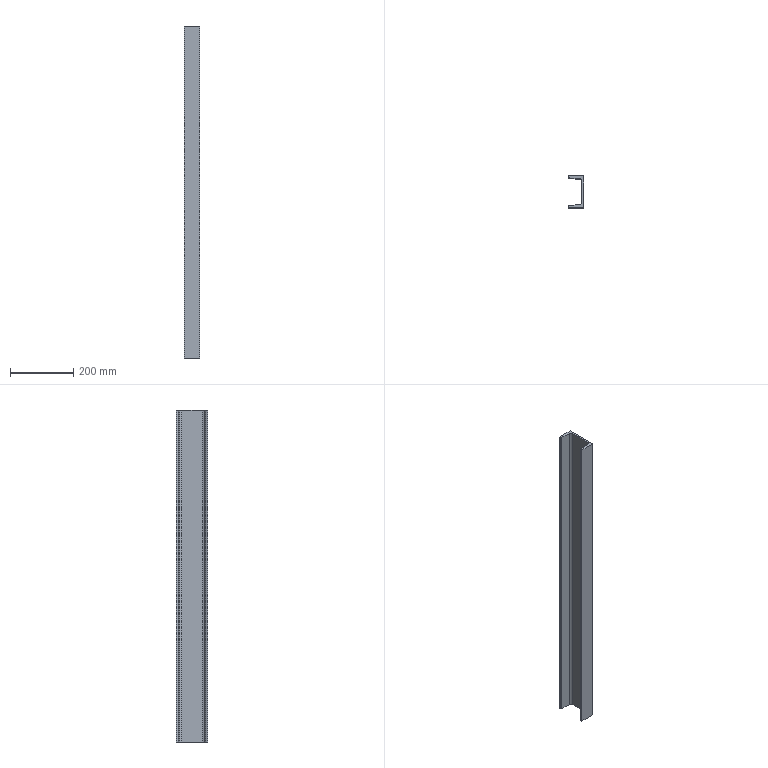Part | SolidWorks | features BaseBody 1 | 1 solid | 14 faces | box 48 x 100 x 1046 mm | volume 1315987 mm3 | plane 10 | cylinder 4 | commonest cylinder face diameters 8.5 x2 17 x2
STEP:
#1=CARTESIAN_POINT('',(2.65,50.,-523.));
#2=VERTEX_POINT('',#1);
#3=CARTESIAN_POINT('',(2.65,-50.,-523.));
#4=VERTEX_POINT('',#3);
#5=CARTESIAN_POINT('',(2.65,50.,-523.));
#6=DIRECTION('',(0.,-1.,0.));
#7=VECTOR('',#6,1000.);
#8=LINE('',#5,#7);
#9=EDGE_CURVE('',#2,#4,#8,.T.);
#10=ORIENTED_EDGE('',*,*,#9,.T.);
#11=CARTESIAN_POINT('',(-45.35,-50.,-523.));
#12=VERTEX_POINT('',#11);
#13=CARTESIAN_POINT('',(2.65,-50.,-523.));
#14=DIRECTION('',(-1.,0.,0.));
#15=VECTOR('',#14,1000.);
#16=LINE('',#13,#15);
#17=EDGE_CURVE('',#4,#12,#16,.T.);
#18=ORIENTED_EDGE('',*,*,#17,.T.);
#19=CARTESIAN_POINT('',(-45.35,-47.266,-523.));
#20=VERTEX_POINT('',#19);
#21=CARTESIAN_POINT('',(-45.35,-47.266,-523.));
#22=DIRECTION('',(0.,-1.,0.));
#23=VECTOR('',#22,1000.);
#24=LINE('',#21,#23);
#25=EDGE_CURVE('',#20,#12,#24,.T.);
#26=ORIENTED_EDGE('',*,*,#25,.F.);
#27=CARTESIAN_POINT('',(-41.423,-43.028,-523.));
#28=VERTEX_POINT('',#27);
#29=CARTESIAN_POINT('',(-41.1,-47.266,-523.));
#30=DIRECTION('',(0.,0.,1.));
#31=DIRECTION('',(1.,0.,0.));
#32=AXIS2_PLACEMENT_3D('',#29,#30,#31);
#33=CIRCLE('',#32,4.25);
#34=EDGE_CURVE('',#28,#20,#33,.T.);
#35=ORIENTED_EDGE('',*,*,#34,.F.);
#36=CARTESIAN_POINT('',(-10.505,-40.675,-523.));
#37=VERTEX_POINT('',#36);
#38=CARTESIAN_POINT('',(-10.505,-40.675,-523.));
#39=DIRECTION('',(-0.9971,-0.07589,0.));
#40=VECTOR('',#39,1000.);
#41=LINE('',#38,#40);
#42=EDGE_CURVE('',#37,#28,#41,.T.);
#43=ORIENTED_EDGE('',*,*,#42,.F.);
#44=CARTESIAN_POINT('',(-2.65,-32.199,-523.));
#45=VERTEX_POINT('',#44);
#46=CARTESIAN_POINT('',(-11.15,-32.199,-523.));
#47=DIRECTION('',(0.,0.,-1.));
#48=DIRECTION('',(-1.,0.,0.));
#49=AXIS2_PLACEMENT_3D('',#46,#47,#48);
#50=CIRCLE('',#49,8.5);
#51=EDGE_CURVE('',#45,#37,#50,.T.);
#52=ORIENTED_EDGE('',*,*,#51,.F.);
#53=CARTESIAN_POINT('',(-2.65,32.199,-523.));
#54=VERTEX_POINT('',#53);
#55=CARTESIAN_POINT('',(-2.65,-32.199,-523.));
#56=DIRECTION('',(0.,1.,0.));
#57=VECTOR('',#56,1000.);
#58=LINE('',#55,#57);
#59=EDGE_CURVE('',#45,#54,#58,.T.);
#60=ORIENTED_EDGE('',*,*,#59,.T.);
#61=CARTESIAN_POINT('',(-10.505,40.675,-523.));
#62=VERTEX_POINT('',#61);
#63=CARTESIAN_POINT('',(-11.15,32.199,-523.));
#64=DIRECTION('',(0.,0.,-1.));
#65=DIRECTION('',(-1.,0.,0.));
#66=AXIS2_PLACEMENT_3D('',#63,#64,#65);
#67=CIRCLE('',#66,8.5);
#68=EDGE_CURVE('',#62,#54,#67,.T.);
#69=ORIENTED_EDGE('',*,*,#68,.F.);
#70=CARTESIAN_POINT('',(-41.423,43.028,-523.));
#71=VERTEX_POINT('',#70);
#72=CARTESIAN_POINT('',(-10.505,40.675,-523.));
#73=DIRECTION('',(-0.9971,0.07589,0.));
#74=VECTOR('',#73,1000.);
#75=LINE('',#72,#74);
#76=EDGE_CURVE('',#62,#71,#75,.T.);
#77=ORIENTED_EDGE('',*,*,#76,.T.);
#78=CARTESIAN_POINT('',(-45.35,47.266,-523.));
#79=VERTEX_POINT('',#78);
#80=CARTESIAN_POINT('',(-41.1,47.266,-523.));
#81=DIRECTION('',(0.,0.,1.));
#82=DIRECTION('',(1.,0.,0.));
#83=AXIS2_PLACEMENT_3D('',#80,#81,#82);
#84=CIRCLE('',#83,4.25);
#85=EDGE_CURVE('',#79,#71,#84,.T.);
#86=ORIENTED_EDGE('',*,*,#85,.F.);
#87=CARTESIAN_POINT('',(-45.35,50.,-523.));
#88=VERTEX_POINT('',#87);
#89=CARTESIAN_POINT('',(-45.35,47.266,-523.));
#90=DIRECTION('',(0.,1.,0.));
#91=VECTOR('',#90,1000.);
#92=LINE('',#89,#91);
#93=EDGE_CURVE('',#79,#88,#92,.T.);
#94=ORIENTED_EDGE('',*,*,#93,.T.);
#95=CARTESIAN_POINT('',(2.65,50.,-523.));
#96=DIRECTION('',(-1.,0.,0.));
#97=VECTOR('',#96,1000.);
#98=LINE('',#95,#97);
#99=EDGE_CURVE('',#2,#88,#98,.T.);
#100=ORIENTED_EDGE('',*,*,#99,.F.);
#101=EDGE_LOOP('',(#10,#18,#26,#35,#43,#52,#60,#69,#77,#86,#94,#100));
#102=FACE_OUTER_BOUND('',#101,.T.);
#103=CARTESIAN_POINT('',(-41.1,-47.266,-523.));
#104=DIRECTION('',(0.,0.,1.));
#105=DIRECTION('',(1.,0.,0.));
#106=AXIS2_PLACEMENT_3D('',#103,#104,#105);
#107=PLANE('',#106);
#108=ADVANCED_FACE('',(#102),#107,.F.);
#109=CARTESIAN_POINT('',(2.65,50.,523.));
#110=VERTEX_POINT('',#109);
#111=CARTESIAN_POINT('',(2.65,-50.,523.));
#112=VERTEX_POINT('',#111);
#113=CARTESIAN_POINT('',(2.65,50.,523.));
#114=DIRECTION('',(0.,-1.,0.));
#115=VECTOR('',#114,1000.);
#116=LINE('',#113,#115);
#117=EDGE_CURVE('',#110,#112,#116,.T.);
#118=ORIENTED_EDGE('',*,*,#117,.F.);
#119=CARTESIAN_POINT('',(-45.35,50.,523.));
#120=VERTEX_POINT('',#119);
#121=CARTESIAN_POINT('',(2.65,50.,523.));
#122=DIRECTION('',(-1.,0.,0.));
#123=VECTOR('',#122,1000.);
#124=LINE('',#121,#123);
#125=EDGE_CURVE('',#110,#120,#124,.T.);
#126=ORIENTED_EDGE('',*,*,#125,.T.);
#127=CARTESIAN_POINT('',(-45.35,47.266,523.));
#128=VERTEX_POINT('',#127);
#129=CARTESIAN_POINT('',(-45.35,47.266,523.));
#130=DIRECTION('',(0.,1.,0.));
#131=VECTOR('',#130,1000.);
#132=LINE('',#129,#131);
#133=EDGE_CURVE('',#128,#120,#132,.T.);
#134=ORIENTED_EDGE('',*,*,#133,.F.);
#135=CARTESIAN_POINT('',(-41.423,43.028,523.));
#136=VERTEX_POINT('',#135);
#137=CARTESIAN_POINT('',(-41.1,47.266,523.));
#138=DIRECTION('',(0.,0.,1.));
#139=DIRECTION('',(1.,0.,0.));
#140=AXIS2_PLACEMENT_3D('',#137,#138,#139);
#141=CIRCLE('',#140,4.25);
#142=EDGE_CURVE('',#128,#136,#141,.T.);
#143=ORIENTED_EDGE('',*,*,#142,.T.);
#144=CARTESIAN_POINT('',(-10.505,40.675,523.));
#145=VERTEX_POINT('',#144);
#146=CARTESIAN_POINT('',(-10.505,40.675,523.));
#147=DIRECTION('',(-0.9971,0.07589,0.));
#148=VECTOR('',#147,1000.);
#149=LINE('',#146,#148);
#150=EDGE_CURVE('',#145,#136,#149,.T.);
#151=ORIENTED_EDGE('',*,*,#150,.F.);
#152=CARTESIAN_POINT('',(-2.65,32.199,523.));
#153=VERTEX_POINT('',#152);
#154=CARTESIAN_POINT('',(-11.15,32.199,523.));
#155=DIRECTION('',(0.,0.,-1.));
#156=DIRECTION('',(-1.,0.,0.));
#157=AXIS2_PLACEMENT_3D('',#154,#155,#156);
#158=CIRCLE('',#157,8.5);
#159=EDGE_CURVE('',#145,#153,#158,.T.);
#160=ORIENTED_EDGE('',*,*,#159,.T.);
#161=CARTESIAN_POINT('',(-2.65,-32.199,523.));
#162=VERTEX_POINT('',#161);
#163=CARTESIAN_POINT('',(-2.65,-32.199,523.));
#164=DIRECTION('',(0.,1.,0.));
#165=VECTOR('',#164,1000.);
#166=LINE('',#163,#165);
#167=EDGE_CURVE('',#162,#153,#166,.T.);
#168=ORIENTED_EDGE('',*,*,#167,.F.);
#169=CARTESIAN_POINT('',(-10.505,-40.675,523.));
#170=VERTEX_POINT('',#169);
#171=CARTESIAN_POINT('',(-11.15,-32.199,523.));
#172=DIRECTION('',(0.,0.,-1.));
#173=DIRECTION('',(-1.,0.,0.));
#174=AXIS2_PLACEMENT_3D('',#171,#172,#173);
#175=CIRCLE('',#174,8.5);
#176=EDGE_CURVE('',#162,#170,#175,.T.);
#177=ORIENTED_EDGE('',*,*,#176,.T.);
#178=CARTESIAN_POINT('',(-41.423,-43.028,523.));
#179=VERTEX_POINT('',#178);
#180=CARTESIAN_POINT('',(-10.505,-40.675,523.));
#181=DIRECTION('',(-0.9971,-0.07589,0.));
#182=VECTOR('',#181,1000.);
#183=LINE('',#180,#182);
#184=EDGE_CURVE('',#170,#179,#183,.T.);
#185=ORIENTED_EDGE('',*,*,#184,.T.);
#186=CARTESIAN_POINT('',(-45.35,-47.266,523.));
#187=VERTEX_POINT('',#186);
#188=CARTESIAN_POINT('',(-41.1,-47.266,523.));
#189=DIRECTION('',(0.,0.,1.));
#190=DIRECTION('',(1.,0.,0.));
#191=AXIS2_PLACEMENT_3D('',#188,#189,#190);
#192=CIRCLE('',#191,4.25);
#193=EDGE_CURVE('',#179,#187,#192,.T.);
#194=ORIENTED_EDGE('',*,*,#193,.T.);
#195=CARTESIAN_POINT('',(-45.35,-50.,523.));
#196=VERTEX_POINT('',#195);
#197=CARTESIAN_POINT('',(-45.35,-47.266,523.));
#198=DIRECTION('',(0.,-1.,0.));
#199=VECTOR('',#198,1000.);
#200=LINE('',#197,#199);
#201=EDGE_CURVE('',#187,#196,#200,.T.);
#202=ORIENTED_EDGE('',*,*,#201,.T.);
#203=CARTESIAN_POINT('',(2.65,-50.,523.));
#204=DIRECTION('',(-1.,0.,0.));
#205=VECTOR('',#204,1000.);
#206=LINE('',#203,#205);
#207=EDGE_CURVE('',#112,#196,#206,.T.);
#208=ORIENTED_EDGE('',*,*,#207,.F.);
#209=EDGE_LOOP('',(#118,#126,#134,#143,#151,#160,#168,#177,#185,#194,#202,#208));
#210=FACE_OUTER_BOUND('',#209,.T.);
#211=CARTESIAN_POINT('',(-41.1,-47.266,523.));
#212=DIRECTION('',(0.,0.,1.));
#213=DIRECTION('',(1.,0.,0.));
#214=AXIS2_PLACEMENT_3D('',#211,#212,#213);
#215=PLANE('',#214);
#216=ADVANCED_FACE('',(#210),#215,.T.);
#217=ORIENTED_EDGE('',*,*,#17,.F.);
#218=CARTESIAN_POINT('',(2.65,-50.,523.));
#219=DIRECTION('',(0.,0.,-1.));
#220=VECTOR('',#219,1000.);
#221=LINE('',#218,#220);
#222=EDGE_CURVE('',#112,#4,#221,.T.);
#223=ORIENTED_EDGE('',*,*,#222,.F.);
#224=ORIENTED_EDGE('',*,*,#207,.T.);
#225=CARTESIAN_POINT('',(-45.35,-50.,523.));
#226=DIRECTION('',(0.,0.,-1.));
#227=VECTOR('',#226,1000.);
#228=LINE('',#225,#227);
#229=EDGE_CURVE('',#196,#12,#228,.T.);
#230=ORIENTED_EDGE('',*,*,#229,.T.);
#231=EDGE_LOOP('',(#217,#223,#224,#230));
#232=FACE_OUTER_BOUND('',#231,.T.);
#233=CARTESIAN_POINT('',(2.65,-50.,523.));
#234=DIRECTION('',(0.,-1.,0.));
#235=DIRECTION('',(0.,0.,-1.));
#236=AXIS2_PLACEMENT_3D('',#233,#234,#235);
#237=PLANE('',#236);
#238=ADVANCED_FACE('',(#232),#237,.T.);
#239=ORIENTED_EDGE('',*,*,#25,.T.);
#240=ORIENTED_EDGE('',*,*,#229,.F.);
#241=ORIENTED_EDGE('',*,*,#201,.F.);
#242=CARTESIAN_POINT('',(-45.35,-47.266,523.));
#243=DIRECTION('',(0.,0.,-1.));
#244=VECTOR('',#243,1000.);
#245=LINE('',#242,#244);
#246=EDGE_CURVE('',#187,#20,#245,.T.);
#247=ORIENTED_EDGE('',*,*,#246,.T.);
#248=EDGE_LOOP('',(#239,#240,#241,#247));
#249=FACE_OUTER_BOUND('',#248,.T.);
#250=CARTESIAN_POINT('',(-45.35,-47.266,523.));
#251=DIRECTION('',(1.,0.,0.));
#252=DIRECTION('',(0.,1.,0.));
#253=AXIS2_PLACEMENT_3D('',#250,#251,#252);
#254=PLANE('',#253);
#255=ADVANCED_FACE('',(#249),#254,.F.);
#256=ORIENTED_EDGE('',*,*,#34,.T.);
#257=ORIENTED_EDGE('',*,*,#246,.F.);
#258=ORIENTED_EDGE('',*,*,#193,.F.);
#259=CARTESIAN_POINT('',(-41.423,-43.028,523.));
#260=DIRECTION('',(0.,0.,-1.));
#261=VECTOR('',#260,1000.);
#262=LINE('',#259,#261);
#263=EDGE_CURVE('',#179,#28,#262,.T.);
#264=ORIENTED_EDGE('',*,*,#263,.T.);
#265=EDGE_LOOP('',(#256,#257,#258,#264));
#266=FACE_OUTER_BOUND('',#265,.T.);
#267=CARTESIAN_POINT('',(-41.1,-47.266,523.));
#268=DIRECTION('',(0.,0.,-1.));
#269=DIRECTION('',(-1.,0.,0.));
#270=AXIS2_PLACEMENT_3D('',#267,#268,#269);
#271=CYLINDRICAL_SURFACE('',#270,4.25);
#272=ADVANCED_FACE('',(#266),#271,.T.);
#273=ORIENTED_EDGE('',*,*,#42,.T.);
#274=ORIENTED_EDGE('',*,*,#263,.F.);
#275=ORIENTED_EDGE('',*,*,#184,.F.);
#276=CARTESIAN_POINT('',(-10.505,-40.675,523.));
#277=DIRECTION('',(0.,0.,-1.));
#278=VECTOR('',#277,1000.);
#279=LINE('',#276,#278);
#280=EDGE_CURVE('',#170,#37,#279,.T.);
#281=ORIENTED_EDGE('',*,*,#280,.T.);
#282=EDGE_LOOP('',(#273,#274,#275,#281));
#283=FACE_OUTER_BOUND('',#282,.T.);
#284=CARTESIAN_POINT('',(-10.505,-40.675,523.));
#285=DIRECTION('',(0.07589,-0.9971,0.));
#286=DIRECTION('',(0.,0.,-1.));
#287=AXIS2_PLACEMENT_3D('',#284,#285,#286);
#288=PLANE('',#287);
#289=ADVANCED_FACE('',(#283),#288,.F.);
#290=ORIENTED_EDGE('',*,*,#51,.T.);
#291=ORIENTED_EDGE('',*,*,#280,.F.);
#292=ORIENTED_EDGE('',*,*,#176,.F.);
#293=CARTESIAN_POINT('',(-2.65,-32.199,523.));
#294=DIRECTION('',(0.,0.,-1.));
#295=VECTOR('',#294,1000.);
#296=LINE('',#293,#295);
#297=EDGE_CURVE('',#162,#45,#296,.T.);
#298=ORIENTED_EDGE('',*,*,#297,.T.);
#299=EDGE_LOOP('',(#290,#291,#292,#298));
#300=FACE_OUTER_BOUND('',#299,.T.);
#301=CARTESIAN_POINT('',(-11.15,-32.199,523.));
#302=DIRECTION('',(0.,0.,-1.));
#303=DIRECTION('',(-1.,0.,0.));
#304=AXIS2_PLACEMENT_3D('',#301,#302,#303);
#305=CYLINDRICAL_SURFACE('',#304,8.5);
#306=ADVANCED_FACE('',(#300),#305,.F.);
#307=ORIENTED_EDGE('',*,*,#59,.F.);
#308=ORIENTED_EDGE('',*,*,#297,.F.);
#309=ORIENTED_EDGE('',*,*,#167,.T.);
#310=CARTESIAN_POINT('',(-2.65,32.199,523.));
#311=DIRECTION('',(0.,0.,-1.));
#312=VECTOR('',#311,1000.);
#313=LINE('',#310,#312);
#314=EDGE_CURVE('',#153,#54,#313,.T.);
#315=ORIENTED_EDGE('',*,*,#314,.T.);
#316=EDGE_LOOP('',(#307,#308,#309,#315));
#317=FACE_OUTER_BOUND('',#316,.T.);
#318=CARTESIAN_POINT('',(-2.65,-32.199,523.));
#319=DIRECTION('',(-1.,0.,0.));
#320=DIRECTION('',(0.,1.,0.));
#321=AXIS2_PLACEMENT_3D('',#318,#319,#320);
#322=PLANE('',#321);
#323=ADVANCED_FACE('',(#317),#322,.T.);
#324=ORIENTED_EDGE('',*,*,#68,.T.);
#325=ORIENTED_EDGE('',*,*,#314,.F.);
#326=ORIENTED_EDGE('',*,*,#159,.F.);
#327=CARTESIAN_POINT('',(-10.505,40.675,523.));
#328=DIRECTION('',(0.,0.,-1.));
#329=VECTOR('',#328,1000.);
#330=LINE('',#327,#329);
#331=EDGE_CURVE('',#145,#62,#330,.T.);
#332=ORIENTED_EDGE('',*,*,#331,.T.);
#333=EDGE_LOOP('',(#324,#325,#326,#332));
#334=FACE_OUTER_BOUND('',#333,.T.);
#335=CARTESIAN_POINT('',(-11.15,32.199,523.));
#336=DIRECTION('',(0.,0.,-1.));
#337=DIRECTION('',(-1.,0.,0.));
#338=AXIS2_PLACEMENT_3D('',#335,#336,#337);
#339=CYLINDRICAL_SURFACE('',#338,8.5);
#340=ADVANCED_FACE('',(#334),#339,.F.);
#341=ORIENTED_EDGE('',*,*,#76,.F.);
#342=ORIENTED_EDGE('',*,*,#331,.F.);
#343=ORIENTED_EDGE('',*,*,#150,.T.);
#344=CARTESIAN_POINT('',(-41.423,43.028,523.));
#345=DIRECTION('',(0.,0.,-1.));
#346=VECTOR('',#345,1000.);
#347=LINE('',#344,#346);
#348=EDGE_CURVE('',#136,#71,#347,.T.);
#349=ORIENTED_EDGE('',*,*,#348,.T.);
#350=EDGE_LOOP('',(#341,#342,#343,#349));
#351=FACE_OUTER_BOUND('',#350,.T.);
#352=CARTESIAN_POINT('',(-10.505,40.675,523.));
#353=DIRECTION('',(-0.07589,-0.9971,0.));
#354=DIRECTION('',(-0.9971,0.07589,0.));
#355=AXIS2_PLACEMENT_3D('',#352,#353,#354);
#356=PLANE('',#355);
#357=ADVANCED_FACE('',(#351),#356,.T.);
#358=ORIENTED_EDGE('',*,*,#85,.T.);
#359=ORIENTED_EDGE('',*,*,#348,.F.);
#360=ORIENTED_EDGE('',*,*,#142,.F.);
#361=CARTESIAN_POINT('',(-45.35,47.266,523.));
#362=DIRECTION('',(0.,0.,-1.));
#363=VECTOR('',#362,1000.);
#364=LINE('',#361,#363);
#365=EDGE_CURVE('',#128,#79,#364,.T.);
#366=ORIENTED_EDGE('',*,*,#365,.T.);
#367=EDGE_LOOP('',(#358,#359,#360,#366));
#368=FACE_OUTER_BOUND('',#367,.T.);
#369=CARTESIAN_POINT('',(-41.1,47.266,523.));
#370=DIRECTION('',(0.,0.,-1.));
#371=DIRECTION('',(-1.,0.,0.));
#372=AXIS2_PLACEMENT_3D('',#369,#370,#371);
#373=CYLINDRICAL_SURFACE('',#372,4.25);
#374=ADVANCED_FACE('',(#368),#373,.T.);
#375=ORIENTED_EDGE('',*,*,#93,.F.);
#376=ORIENTED_EDGE('',*,*,#365,.F.);
#377=ORIENTED_EDGE('',*,*,#133,.T.);
#378=CARTESIAN_POINT('',(-45.35,50.,523.));
#379=DIRECTION('',(0.,0.,-1.));
#380=VECTOR('',#379,1000.);
#381=LINE('',#378,#380);
#382=EDGE_CURVE('',#120,#88,#381,.T.);
#383=ORIENTED_EDGE('',*,*,#382,.T.);
#384=EDGE_LOOP('',(#375,#376,#377,#383));
#385=FACE_OUTER_BOUND('',#384,.T.);
#386=CARTESIAN_POINT('',(-45.35,47.266,523.));
#387=DIRECTION('',(-1.,0.,0.));
#388=DIRECTION('',(0.,1.,0.));
#389=AXIS2_PLACEMENT_3D('',#386,#387,#388);
#390=PLANE('',#389);
#391=ADVANCED_FACE('',(#385),#390,.T.);
#392=ORIENTED_EDGE('',*,*,#99,.T.);
#393=ORIENTED_EDGE('',*,*,#382,.F.);
#394=ORIENTED_EDGE('',*,*,#125,.F.);
#395=CARTESIAN_POINT('',(2.65,50.,523.));
#396=DIRECTION('',(0.,0.,-1.));
#397=VECTOR('',#396,1000.);
#398=LINE('',#395,#397);
#399=EDGE_CURVE('',#110,#2,#398,.T.);
#400=ORIENTED_EDGE('',*,*,#399,.T.);
#401=EDGE_LOOP('',(#392,#393,#394,#400));
#402=FACE_OUTER_BOUND('',#401,.T.);
#403=CARTESIAN_POINT('',(2.65,50.,523.));
#404=DIRECTION('',(0.,-1.,0.));
#405=DIRECTION('',(0.,0.,-1.));
#406=AXIS2_PLACEMENT_3D('',#403,#404,#405);
#407=PLANE('',#406);
#408=ADVANCED_FACE('',(#402),#407,.F.);
#409=ORIENTED_EDGE('',*,*,#9,.F.);
#410=ORIENTED_EDGE('',*,*,#399,.F.);
#411=ORIENTED_EDGE('',*,*,#117,.T.);
#412=ORIENTED_EDGE('',*,*,#222,.T.);
#413=EDGE_LOOP('',(#409,#410,#411,#412));
#414=FACE_OUTER_BOUND('',#413,.T.);
#415=CARTESIAN_POINT('',(2.65,50.,523.));
#416=DIRECTION('',(1.,0.,0.));
#417=DIRECTION('',(0.,-1.,0.));
#418=AXIS2_PLACEMENT_3D('',#415,#416,#417);
#419=PLANE('',#418);
#420=ADVANCED_FACE('',(#414),#419,.T.);
#421=CLOSED_SHELL('',(#108,#216,#238,#255,#272,#289,#306,#323,#340,#357,#374,#391,#408,#420));
#422=MANIFOLD_SOLID_BREP('',#421);
#423=CARTESIAN_POINT('',(0.,0.,0.));
#424=DIRECTION('',(0.,0.,1.));
#425=DIRECTION('',(1.,0.,0.));
#426=AXIS2_PLACEMENT_3D('',#423,#424,#425);
#427=(LENGTH_UNIT()NAMED_UNIT(*)SI_UNIT(.MILLI.,.METRE.));
#428=UNCERTAINTY_MEASURE_WITH_UNIT(LENGTH_MEASURE(0.00001),#427,'','');
#429=(NAMED_UNIT(*)PLANE_ANGLE_UNIT()SI_UNIT($,.RADIAN.));
#430=(NAMED_UNIT(*)SI_UNIT($,.STERADIAN.)SOLID_ANGLE_UNIT());
#431=(GEOMETRIC_REPRESENTATION_CONTEXT(3)GLOBAL_UNCERTAINTY_ASSIGNED_CONTEXT((#428))GLOBAL_UNIT_ASSIGNED_CONTEXT((#427,#429,#430))REPRESENTATION_CONTEXT('',''));
#432=ADVANCED_BREP_SHAPE_REPRESENTATION('',(#422,#426),#431);